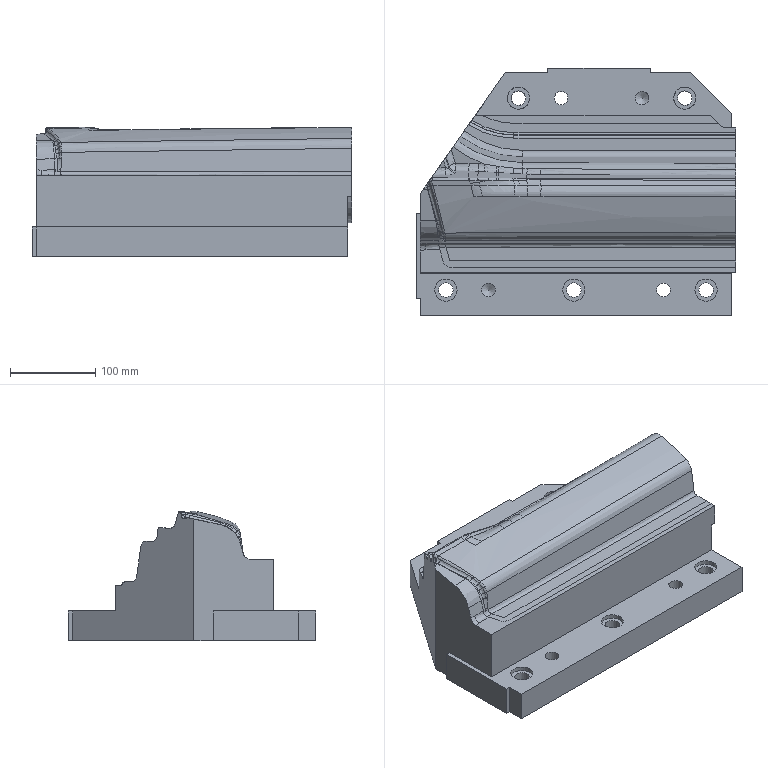Part | NX | features solid 2 | 1 solid | 155 faces | box 375 x 290 x 151.986 mm | volume 6900853 mm3 | spline 105 | plane 34 | cylinder 14 | cone 2 | commonest cylinder face diameters 17 x5 26 x5 16 x4